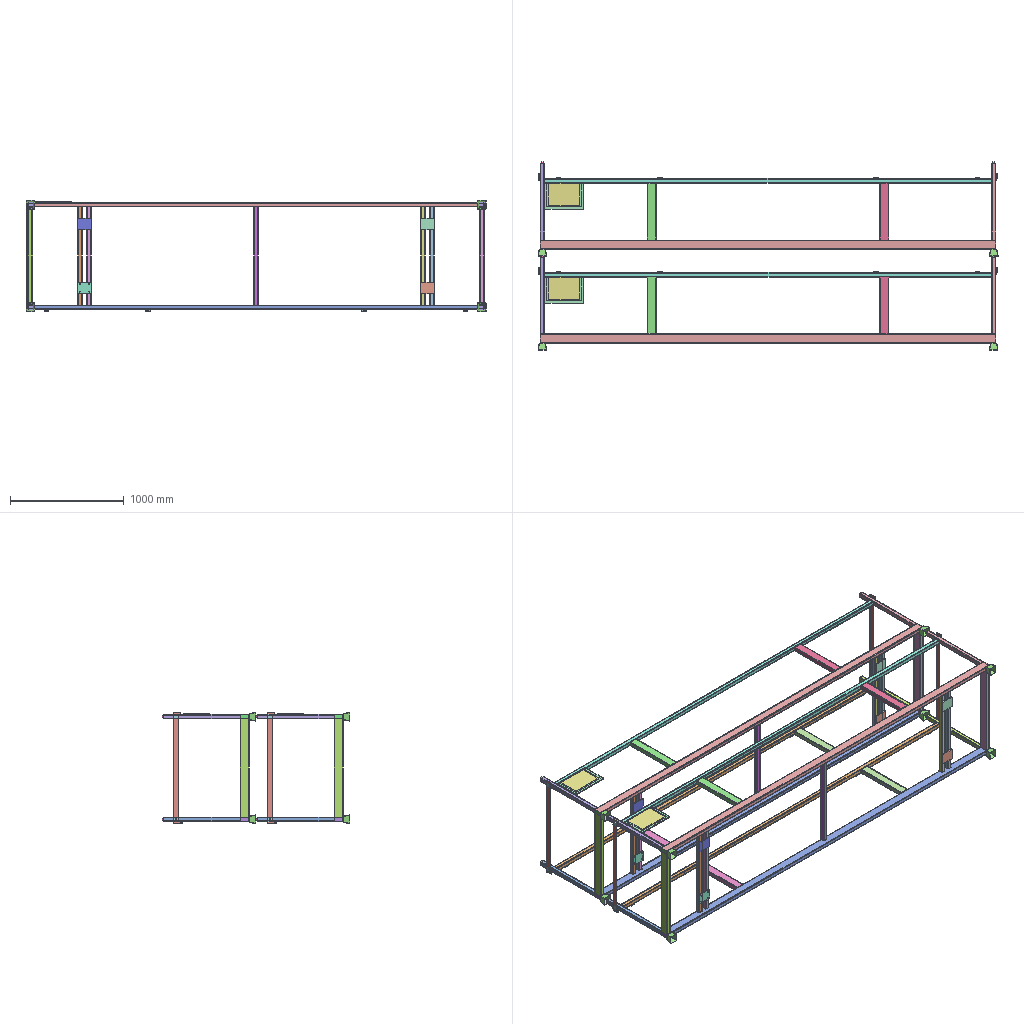Assembly | SolidWorks | 11 different items | 98 placed | box 4036 x 1648 x 980 mm
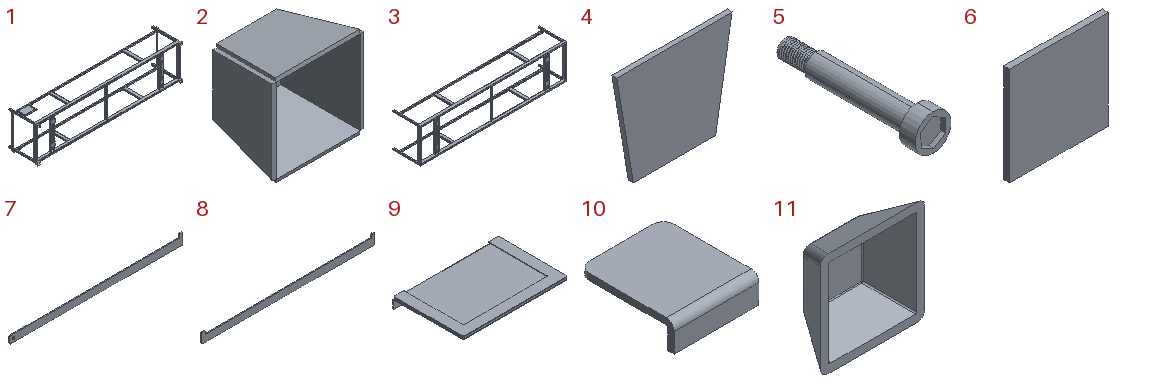Parts list (item | name | quantity | parent item | size | volume | features):
1 | (subassembly) | x2 | - | 4036 x 824.161 x 980 mm | 15514087 mm3 | features ReferencePattern 11, MirrorCompFeat 6, LocalLPattern 2
2 | (subassembly) | x8 | in 1 | 75.916 x 59.661 x 75.916 mm | 61500 mm3 | features ReferencePattern 3, MirrorCompFeat 2
3 | - | x2 | in 1 | 4000 x 750 x 940 mm | 14483541 mm3 | features WeldCornerFeat 3, ICE 2, MirrorSolid 2, WeldMemberFeat 2, 3DProfileFeature 1, Cut 1, EndCap 1, Fillet 1, HoleWzd 1, MoveCopyBody 1, WeldmentFeature 1
4 | - | x40 | in 2 | 70 x 3 x 60 mm | 10800 mm3 | features Extrusion 1
5 | - | x4 | in 1 | 16 x 65.25 x 16 mm | 5296 mm3 | features ICE 3, Extrusion 1, SweepThread 1
6 | - | x8 | in 2 | 50 x 3 x 50 mm | 7500 mm3 | features Extrusion 1
7 | - | x4 | in 1 | 960 x 5 x 60 mm | 193100 mm3 | features ICE 2, Fillet 1, FlatPattern 1, SMBaseFlange 1, SheetMetal 1
8 | - | x4 | in 1 | 980 x 5 x 60 mm | 199439 mm3 | features ICE 3, Fillet 2, FlatPattern 1, SMBaseFlange 1, SheetMetal 1
9 | - | x2 | in 1 | 342 x 230 x 38 mm | 314217 mm3 | features Fillet 4, ICE 2, EdgeFlange 1, FlatPattern 1, SMBaseFlange 1, SheetMetal 1
10 | - | x16 | in 1 | 40 x 45 x 13 mm | 6453 mm3 | features EdgeFlange 1, Fillet 1, FlatPattern 1, SMBaseFlange 1, SheetMetal 1
11 | - | x8 | in 1 | 37 x 15 x 37 mm | 4957 mm3 | features Extrusion 1, Fillet 1, Shell 1
Mates (type | each side: item.copy, entity, surface, feature):
In the top assembly
Coincident | 3.1 face plane GB/T 6728-2002 Rectangular hollow section 080X40X3 | 3.2 face plane GB/T 6728-2002 Rectangular hollow section 080X40X3 | 2 times
In subassembly 1
Coincident | 3.3 face plane GB/T 6728-2002 Rectangular hollow section 080X40X3 | 6.1 face plane Boss-Extrude1
Coincident | 3.3 face plane GB/T 6728-2002 Square hollow section 40×3 | 11.1 face plane Boss-Extrude1
DistanceDim | 3.3 face plane GB/T 6728-2002 Square hollow section 40×3 | 11.1 edge
DistanceDim | 11.1 edge | 3.3 face plane GB/T 6728-2002 Square hollow section 40×3
DistanceDim | 4.1 edge | 3.3 face plane GB/T 6728-2002 Rectangular hollow section 080X40X3
DistanceDim | 3.3 edge | 4.2 edge
Concentric | 3.3 face cylinder Cut-Extrude2 | 7.1 face cylinder Cut-Extrude1
Coincident | 3.3 face plane GB/T 6728-2002 Square hollow section 40×3 | 7.1 face plane Base-Flange1
Concentric | 3.3 face cylinder Cut-Extrude2 | 5.1 face cylinder Boss-Extrude3
Coincident | 3.3 face plane GB/T 6728-2002 Square hollow section 40×3 | 10.1 face plane Base-Flange1 | 3 times
Concentric | 3.3 face cylinder Cut-Extrude2 | 7.2 face cylinder Cut-Extrude1
Coincident | 3.3 face plane GB/T 6728-2002 Square hollow section 40×3 | 7.2 face plane Base-Flange1
Concentric | 3.3 face cylinder Cut-Extrude2 | 5.2 face cylinder Boss-Extrude3
DistanceDim | 7.2 face plane Base-Flange1 | 5.2 face plane Boss-Extrude1
DistanceDim | 5.1 face plane Boss-Extrude1 | 7.1 face plane Base-Flange1
Parallel | 7.1 face plane Base-Flange1 | 10.1 face plane Base-Flange1
Parallel | 7.2 face plane Base-Flange1 | 10.2 face plane Edge-Flange1
Coincident | 3.3 face plane GB/T 6728-2002 Square hollow section 40×3 | 9.1 face plane Base-Flange1 | 2 times
Coincident | 3.3 face plane GB/T 6728-2002 Square hollow section 40×3 | 9.1 face plane Edge-Flange1
Coincident | 3.3 edge | 10.3 face plane Base-Flange1
Coincident | 3.3 face plane GB/T 6728-2002 Square hollow section 40×3 | 10.3 face plane Base-Flange1
DistanceDim | 10.3 face plane Edge-Flange1 | 3.3 face plane GB/T 6728-2002 Square hollow section 40×3
Coincident | 3.3 face plane GB/T 6728-2002 Square hollow section 40×3 | 10.4 face plane Base-Flange1
Coincident | 3.3 edge | 10.4 face plane Base-Flange1
DistanceDim | 10.4 face plane Edge-Flange1 | 3.3 face plane GB/T 6728-2002 Square hollow section 40×3
Coincident | 3.3 face plane GB/T 6728-2002 Square hollow section 40×3 | 8.1 face plane Base-Flange1
Width | 8.1 face plane Base-Flange1 | 8.1 face plane Base-Flange1 | 3.3 face plane GB/T 6728-2002 Square hollow section 40×3 | 3.3 face plane GB/T 6728-2002 Square hollow section 40×3
Coincident | 10.2 face plane Base-Flange1 | 8.1 face plane Base-Flange1
Coincident | 10.5 face plane Edge-Flange1 | 8.2 face plane Base-Flange1
Width | 8.2 face plane Base-Flange1 | 8.2 face plane Base-Flange1 | 3.3 face plane GB/T 6728-2002 Square hollow section 40×3 | 3.3 face plane GB/T 6728-2002 Square hollow section 40×3
Coincident | 10.5 face plane Base-Flange1 | 8.2 face plane Base-Flange1
In subassembly 2
Coincident | 6.2 edge | 4.3 edge
Coincident | 6.2 edge | 4.4 edge
Coincident | 4.3 edge | 4.4 edge